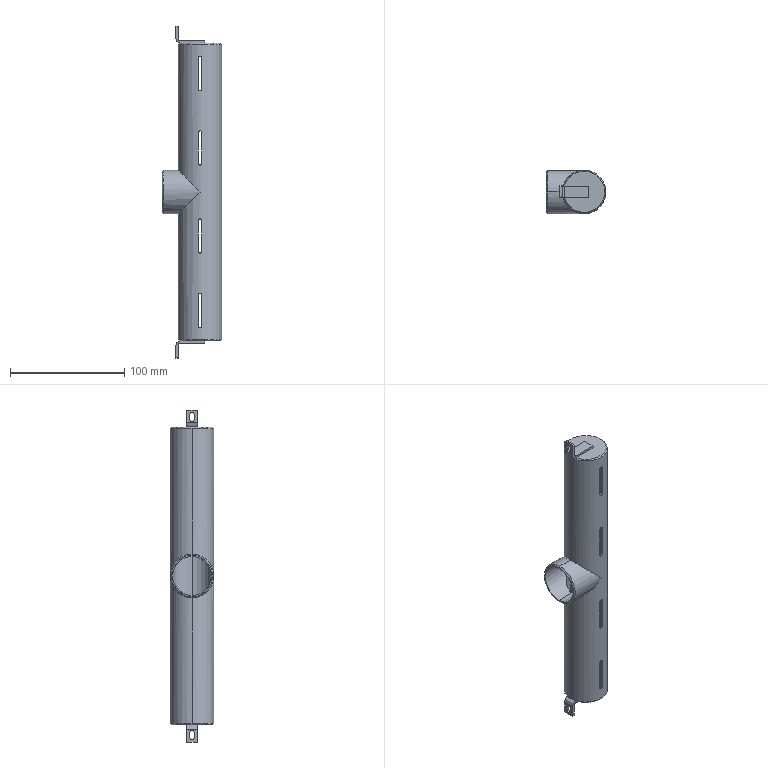Part | SolidWorks | features Fillet 4, ICE 4, Chamfer 3, MirrorPattern 2, Extrusion 1, Shell 1 | 1 solid | 91 faces | box 52 x 38 x 290 mm | volume 64495 mm3 | plane 43 | cylinder 40 | cone 6 | spline 2 | commonest cylinder face diameters 3 x24 3.5 x6 34 x4 38 x4 4 x2